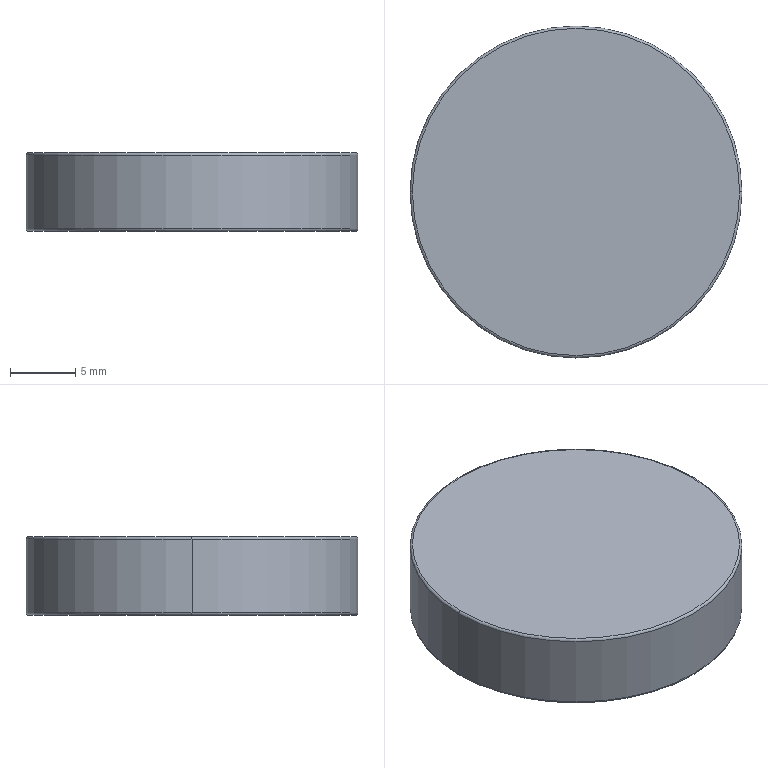Part | STEP file | reflective wave plate-LPM10-532P-HP.step.STEP | 1 solid | 8 faces | box 25.4 x 25.4 x 6 mm | volume 3039 mm3 | torus 4 | cylinder 2 | plane 2 | commonest cylinder face diameters 25.4 x2
STEP:
#1=CARTESIAN_POINT('',(-12.7,0.,5.82));
#2=VERTEX_POINT('',#1);
#3=CARTESIAN_POINT('',(12.7,0.,5.82));
#4=VERTEX_POINT('',#3);
#5=CARTESIAN_POINT('',(0.,0.,5.82));
#6=DIRECTION('',(0.,0.,-1.));
#7=DIRECTION('',(1.,0.,0.));
#8=AXIS2_PLACEMENT_3D('',#5,#6,#7);
#9=CIRCLE('',#8,12.7);
#10=EDGE_CURVE('',#2,#4,#9,.T.);
#11=ORIENTED_EDGE('',*,*,#10,.F.);
#12=CARTESIAN_POINT('',(-12.52,0.,6.));
#13=VERTEX_POINT('',#12);
#14=CARTESIAN_POINT('',(-12.52,0.,5.82));
#15=DIRECTION('',(0.,1.,0.));
#16=DIRECTION('',(-1.,0.,0.));
#17=AXIS2_PLACEMENT_3D('',#14,#15,#16);
#18=CIRCLE('',#17,0.18);
#19=EDGE_CURVE('',#2,#13,#18,.T.);
#20=ORIENTED_EDGE('',*,*,#19,.T.);
#21=CARTESIAN_POINT('',(12.52,0.,6.));
#22=VERTEX_POINT('',#21);
#23=CARTESIAN_POINT('',(0.,0.,6.));
#24=DIRECTION('',(0.,0.,1.));
#25=DIRECTION('',(1.,0.,0.));
#26=AXIS2_PLACEMENT_3D('',#23,#24,#25);
#27=CIRCLE('',#26,12.52);
#28=EDGE_CURVE('',#22,#13,#27,.T.);
#29=ORIENTED_EDGE('',*,*,#28,.F.);
#30=CARTESIAN_POINT('',(12.52,0.,5.82));
#31=DIRECTION('',(0.,-1.,0.));
#32=DIRECTION('',(0.,0.,-1.));
#33=AXIS2_PLACEMENT_3D('',#30,#31,#32);
#34=CIRCLE('',#33,0.18);
#35=EDGE_CURVE('',#4,#22,#34,.T.);
#36=ORIENTED_EDGE('',*,*,#35,.F.);
#37=EDGE_LOOP('',(#11,#20,#29,#36));
#38=FACE_OUTER_BOUND('',#37,.T.);
#39=CARTESIAN_POINT('',(0.,0.,5.82));
#40=DIRECTION('',(0.,0.,1.));
#41=DIRECTION('',(1.,0.,0.));
#42=AXIS2_PLACEMENT_3D('',#39,#40,#41);
#43=TOROIDAL_SURFACE('',#42,12.52,0.18);
#44=ADVANCED_FACE('',(#38),#43,.T.);
#45=CARTESIAN_POINT('',(-12.52,0.,0.));
#46=VERTEX_POINT('',#45);
#47=CARTESIAN_POINT('',(12.52,0.,0.));
#48=VERTEX_POINT('',#47);
#49=CARTESIAN_POINT('',(0.,0.,0.));
#50=DIRECTION('',(0.,0.,-1.));
#51=DIRECTION('',(1.,0.,0.));
#52=AXIS2_PLACEMENT_3D('',#49,#50,#51);
#53=CIRCLE('',#52,12.52);
#54=EDGE_CURVE('',#46,#48,#53,.T.);
#55=ORIENTED_EDGE('',*,*,#54,.F.);
#56=CARTESIAN_POINT('',(-12.7,0.,0.18));
#57=VERTEX_POINT('',#56);
#58=CARTESIAN_POINT('',(-12.52,0.,0.18));
#59=DIRECTION('',(0.,1.,0.));
#60=DIRECTION('',(-1.,0.,0.));
#61=AXIS2_PLACEMENT_3D('',#58,#59,#60);
#62=CIRCLE('',#61,0.18);
#63=EDGE_CURVE('',#46,#57,#62,.T.);
#64=ORIENTED_EDGE('',*,*,#63,.T.);
#65=CARTESIAN_POINT('',(12.7,0.,0.18));
#66=VERTEX_POINT('',#65);
#67=CARTESIAN_POINT('',(0.,0.,0.18));
#68=DIRECTION('',(0.,0.,1.));
#69=DIRECTION('',(1.,0.,0.));
#70=AXIS2_PLACEMENT_3D('',#67,#68,#69);
#71=CIRCLE('',#70,12.7);
#72=EDGE_CURVE('',#66,#57,#71,.T.);
#73=ORIENTED_EDGE('',*,*,#72,.F.);
#74=CARTESIAN_POINT('',(12.52,0.,0.18));
#75=DIRECTION('',(0.,-1.,0.));
#76=DIRECTION('',(0.,0.,-1.));
#77=AXIS2_PLACEMENT_3D('',#74,#75,#76);
#78=CIRCLE('',#77,0.18);
#79=EDGE_CURVE('',#48,#66,#78,.T.);
#80=ORIENTED_EDGE('',*,*,#79,.F.);
#81=EDGE_LOOP('',(#55,#64,#73,#80));
#82=FACE_OUTER_BOUND('',#81,.T.);
#83=CARTESIAN_POINT('',(0.,0.,0.18));
#84=DIRECTION('',(0.,0.,1.));
#85=DIRECTION('',(1.,0.,0.));
#86=AXIS2_PLACEMENT_3D('',#83,#84,#85);
#87=TOROIDAL_SURFACE('',#86,12.52,0.18);
#88=ADVANCED_FACE('',(#82),#87,.T.);
#89=ORIENTED_EDGE('',*,*,#10,.T.);
#90=CARTESIAN_POINT('',(12.7,0.,6.));
#91=DIRECTION('',(0.,0.,-1.));
#92=VECTOR('',#91,1000.);
#93=LINE('',#90,#92);
#94=EDGE_CURVE('',#4,#66,#93,.T.);
#95=ORIENTED_EDGE('',*,*,#94,.T.);
#96=ORIENTED_EDGE('',*,*,#72,.T.);
#97=CARTESIAN_POINT('',(-12.7,0.,6.));
#98=DIRECTION('',(0.,0.,-1.));
#99=VECTOR('',#98,1000.);
#100=LINE('',#97,#99);
#101=EDGE_CURVE('',#2,#57,#100,.T.);
#102=ORIENTED_EDGE('',*,*,#101,.F.);
#103=EDGE_LOOP('',(#89,#95,#96,#102));
#104=FACE_OUTER_BOUND('',#103,.T.);
#105=CARTESIAN_POINT('',(0.,0.,6.));
#106=DIRECTION('',(0.,0.,-1.));
#107=DIRECTION('',(-1.,0.,0.));
#108=AXIS2_PLACEMENT_3D('',#105,#106,#107);
#109=CYLINDRICAL_SURFACE('',#108,12.7);
#110=ADVANCED_FACE('',(#104),#109,.T.);
#111=ORIENTED_EDGE('',*,*,#94,.F.);
#112=CARTESIAN_POINT('',(0.,0.,5.82));
#113=DIRECTION('',(0.,0.,-1.));
#114=DIRECTION('',(1.,0.,0.));
#115=AXIS2_PLACEMENT_3D('',#112,#113,#114);
#116=CIRCLE('',#115,12.7);
#117=EDGE_CURVE('',#4,#2,#116,.T.);
#118=ORIENTED_EDGE('',*,*,#117,.T.);
#119=ORIENTED_EDGE('',*,*,#101,.T.);
#120=CARTESIAN_POINT('',(0.,0.,0.18));
#121=DIRECTION('',(0.,0.,1.));
#122=DIRECTION('',(1.,0.,0.));
#123=AXIS2_PLACEMENT_3D('',#120,#121,#122);
#124=CIRCLE('',#123,12.7);
#125=EDGE_CURVE('',#57,#66,#124,.T.);
#126=ORIENTED_EDGE('',*,*,#125,.T.);
#127=EDGE_LOOP('',(#111,#118,#119,#126));
#128=FACE_OUTER_BOUND('',#127,.T.);
#129=CARTESIAN_POINT('',(0.,0.,6.));
#130=DIRECTION('',(0.,0.,-1.));
#131=DIRECTION('',(-1.,0.,0.));
#132=AXIS2_PLACEMENT_3D('',#129,#130,#131);
#133=CYLINDRICAL_SURFACE('',#132,12.7);
#134=ADVANCED_FACE('',(#128),#133,.T.);
#135=ORIENTED_EDGE('',*,*,#28,.T.);
#136=CARTESIAN_POINT('',(0.,0.,6.));
#137=DIRECTION('',(0.,0.,1.));
#138=DIRECTION('',(1.,0.,0.));
#139=AXIS2_PLACEMENT_3D('',#136,#137,#138);
#140=CIRCLE('',#139,12.52);
#141=EDGE_CURVE('',#13,#22,#140,.T.);
#142=ORIENTED_EDGE('',*,*,#141,.T.);
#143=EDGE_LOOP('',(#135,#142));
#144=FACE_OUTER_BOUND('',#143,.T.);
#145=CARTESIAN_POINT('',(0.,0.,6.));
#146=DIRECTION('',(0.,0.,1.));
#147=DIRECTION('',(1.,0.,0.));
#148=AXIS2_PLACEMENT_3D('',#145,#146,#147);
#149=PLANE('',#148);
#150=ADVANCED_FACE('',(#144),#149,.T.);
#151=CARTESIAN_POINT('',(0.,0.,0.));
#152=DIRECTION('',(0.,0.,-1.));
#153=DIRECTION('',(1.,0.,0.));
#154=AXIS2_PLACEMENT_3D('',#151,#152,#153);
#155=CIRCLE('',#154,12.52);
#156=EDGE_CURVE('',#48,#46,#155,.T.);
#157=ORIENTED_EDGE('',*,*,#156,.T.);
#158=ORIENTED_EDGE('',*,*,#54,.T.);
#159=EDGE_LOOP('',(#157,#158));
#160=FACE_OUTER_BOUND('',#159,.T.);
#161=CARTESIAN_POINT('',(0.,0.,0.));
#162=DIRECTION('',(0.,0.,1.));
#163=DIRECTION('',(1.,0.,0.));
#164=AXIS2_PLACEMENT_3D('',#161,#162,#163);
#165=PLANE('',#164);
#166=ADVANCED_FACE('',(#160),#165,.F.);
#167=ORIENTED_EDGE('',*,*,#63,.F.);
#168=ORIENTED_EDGE('',*,*,#156,.F.);
#169=ORIENTED_EDGE('',*,*,#79,.T.);
#170=ORIENTED_EDGE('',*,*,#125,.F.);
#171=EDGE_LOOP('',(#167,#168,#169,#170));
#172=FACE_OUTER_BOUND('',#171,.T.);
#173=CARTESIAN_POINT('',(0.,0.,0.18));
#174=DIRECTION('',(0.,0.,1.));
#175=DIRECTION('',(1.,0.,0.));
#176=AXIS2_PLACEMENT_3D('',#173,#174,#175);
#177=TOROIDAL_SURFACE('',#176,12.52,0.18);
#178=ADVANCED_FACE('',(#172),#177,.T.);
#179=ORIENTED_EDGE('',*,*,#19,.F.);
#180=ORIENTED_EDGE('',*,*,#117,.F.);
#181=ORIENTED_EDGE('',*,*,#35,.T.);
#182=ORIENTED_EDGE('',*,*,#141,.F.);
#183=EDGE_LOOP('',(#179,#180,#181,#182));
#184=FACE_OUTER_BOUND('',#183,.T.);
#185=CARTESIAN_POINT('',(0.,0.,5.82));
#186=DIRECTION('',(0.,0.,1.));
#187=DIRECTION('',(1.,0.,0.));
#188=AXIS2_PLACEMENT_3D('',#185,#186,#187);
#189=TOROIDAL_SURFACE('',#188,12.52,0.18);
#190=ADVANCED_FACE('',(#184),#189,.T.);
#191=CLOSED_SHELL('',(#44,#88,#110,#134,#150,#166,#178,#190));
#192=MANIFOLD_SOLID_BREP('',#191);
#193=CARTESIAN_POINT('',(0.,0.,0.));
#194=DIRECTION('',(0.,0.,1.));
#195=DIRECTION('',(1.,0.,0.));
#196=AXIS2_PLACEMENT_3D('',#193,#194,#195);
#197=(LENGTH_UNIT()NAMED_UNIT(*)SI_UNIT(.MILLI.,.METRE.));
#198=UNCERTAINTY_MEASURE_WITH_UNIT(LENGTH_MEASURE(0.00001),#197,'','');
#199=(NAMED_UNIT(*)PLANE_ANGLE_UNIT()SI_UNIT($,.RADIAN.));
#200=(NAMED_UNIT(*)SI_UNIT($,.STERADIAN.)SOLID_ANGLE_UNIT());
#201=(GEOMETRIC_REPRESENTATION_CONTEXT(3)GLOBAL_UNCERTAINTY_ASSIGNED_CONTEXT((#198))GLOBAL_UNIT_ASSIGNED_CONTEXT((#197,#199,#200))REPRESENTATION_CONTEXT('',''));
#202=ADVANCED_BREP_SHAPE_REPRESENTATION('',(#192,#196),#201);